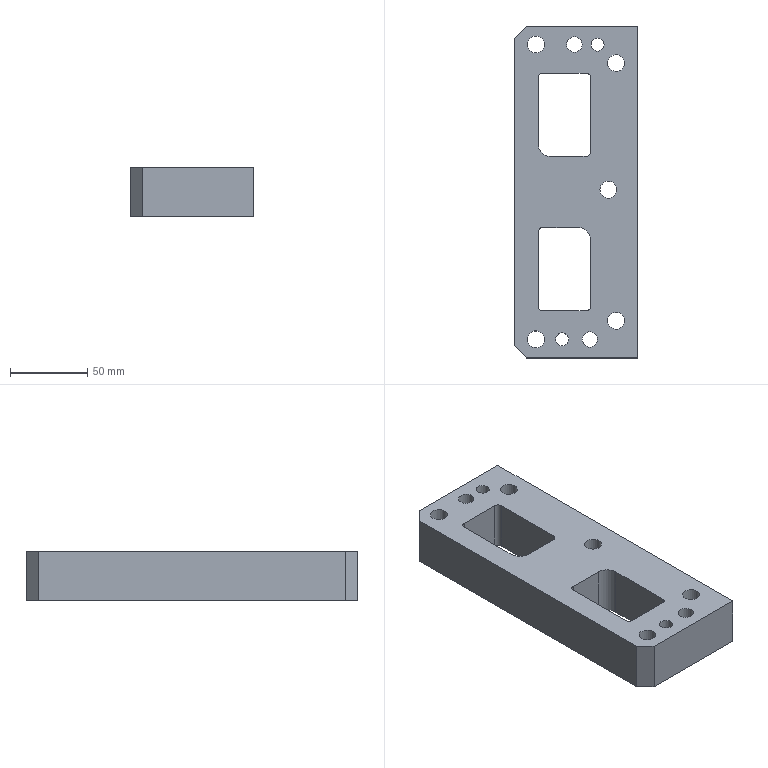Part | STEP file | lll_id3558_x_t | 1 solid | 43 faces | box 80 x 215 x 32 mm | volume 399653 mm3 | cylinder 22 | plane 21 | commonest cylinder face diameters 6 x6 11 x5 17 x5 8.506 x2 10 x2 16 x2
STEP:
#1=CARTESIAN_POINT('',(3684.747,-95.5,60.5));
#2=VERTEX_POINT('',#1);
#3=CARTESIAN_POINT('',(3689.,-95.5,60.5));
#4=DIRECTION('',(0.,0.,1.));
#5=DIRECTION('',(-1.,0.,0.));
#6=AXIS2_PLACEMENT_3D('',#3,#4,#5);
#7=CIRCLE('',#6,4.253);
#8=EDGE_CURVE('',#2,#2,#7,.T.);
#9=ORIENTED_EDGE('',*,*,#8,.T.);
#10=EDGE_LOOP('',(#9));
#11=FACE_BOUND('',#10,.T.);
#12=CARTESIAN_POINT('',(3732.5,-83.5,60.5));
#13=VERTEX_POINT('',#12);
#14=CARTESIAN_POINT('',(3724.,-83.5,60.5));
#15=DIRECTION('',(0.,0.,1.));
#16=DIRECTION('',(1.,0.,0.));
#17=AXIS2_PLACEMENT_3D('',#14,#15,#16);
#18=CIRCLE('',#17,8.5);
#19=EDGE_CURVE('',#13,#13,#18,.T.);
#20=ORIENTED_EDGE('',*,*,#19,.T.);
#21=EDGE_LOOP('',(#20));
#22=FACE_BOUND('',#21,.T.);
#23=CARTESIAN_POINT('',(3680.5,-95.5,60.5));
#24=VERTEX_POINT('',#23);
#25=CARTESIAN_POINT('',(3672.,-95.5,60.5));
#26=DIRECTION('',(0.,0.,1.));
#27=DIRECTION('',(1.,0.,0.));
#28=AXIS2_PLACEMENT_3D('',#25,#26,#27);
#29=CIRCLE('',#28,8.5);
#30=EDGE_CURVE('',#24,#24,#29,.T.);
#31=ORIENTED_EDGE('',*,*,#30,.T.);
#32=EDGE_LOOP('',(#31));
#33=FACE_BOUND('',#32,.T.);
#34=CARTESIAN_POINT('',(3666.,-107.5,60.5));
#35=VERTEX_POINT('',#34);
#36=CARTESIAN_POINT('',(3738.,-107.5,60.5));
#37=VERTEX_POINT('',#36);
#38=CARTESIAN_POINT('',(3700.5,-107.5,60.5));
#39=DIRECTION('',(1.,0.,0.));
#40=VECTOR('',#39,1.);
#41=LINE('',#38,#40);
#42=EDGE_CURVE('',#35,#37,#41,.T.);
#43=ORIENTED_EDGE('',*,*,#42,.F.);
#44=CARTESIAN_POINT('',(3658.,-99.5,60.5));
#45=VERTEX_POINT('',#44);
#46=CARTESIAN_POINT('',(3633.5,-75.,60.5));
#47=DIRECTION('',(-0.7071,0.7071,0.));
#48=VECTOR('',#47,1.);
#49=LINE('',#46,#48);
#50=EDGE_CURVE('',#35,#45,#49,.T.);
#51=ORIENTED_EDGE('',*,*,#50,.T.);
#52=CARTESIAN_POINT('',(3658.,99.5,60.5));
#53=VERTEX_POINT('',#52);
#54=CARTESIAN_POINT('',(3658.,0.00007612,60.5));
#55=DIRECTION('',(0.,-1.,0.));
#56=VECTOR('',#55,1.);
#57=LINE('',#54,#56);
#58=EDGE_CURVE('',#53,#45,#57,.T.);
#59=ORIENTED_EDGE('',*,*,#58,.F.);
#60=CARTESIAN_POINT('',(3666.,107.5,60.5));
#61=VERTEX_POINT('',#60);
#62=CARTESIAN_POINT('',(3633.5,75.,60.5));
#63=DIRECTION('',(0.7071,0.7071,0.));
#64=VECTOR('',#63,1.);
#65=LINE('',#62,#64);
#66=EDGE_CURVE('',#53,#61,#65,.T.);
#67=ORIENTED_EDGE('',*,*,#66,.T.);
#68=CARTESIAN_POINT('',(3738.,107.5,60.5));
#69=VERTEX_POINT('',#68);
#70=CARTESIAN_POINT('',(3700.5,107.5,60.5));
#71=DIRECTION('',(-1.,0.,0.));
#72=VECTOR('',#71,1.);
#73=LINE('',#70,#72);
#74=EDGE_CURVE('',#69,#61,#73,.T.);
#75=ORIENTED_EDGE('',*,*,#74,.F.);
#76=CARTESIAN_POINT('',(3738.,0.00007612,60.5));
#77=DIRECTION('',(0.,1.,0.));
#78=VECTOR('',#77,1.);
#79=LINE('',#76,#78);
#80=EDGE_CURVE('',#37,#69,#79,.T.);
#81=ORIENTED_EDGE('',*,*,#80,.F.);
#82=EDGE_LOOP('',(#43,#51,#59,#67,#75,#81));
#83=FACE_BOUND('',#82,.T.);
#84=CARTESIAN_POINT('',(3732.5,83.5,60.5));
#85=VERTEX_POINT('',#84);
#86=CARTESIAN_POINT('',(3724.,83.5,60.5));
#87=DIRECTION('',(0.,0.,1.));
#88=DIRECTION('',(1.,0.,0.));
#89=AXIS2_PLACEMENT_3D('',#86,#87,#88);
#90=CIRCLE('',#89,8.5);
#91=EDGE_CURVE('',#85,#85,#90,.T.);
#92=ORIENTED_EDGE('',*,*,#91,.T.);
#93=EDGE_LOOP('',(#92));
#94=FACE_BOUND('',#93,.T.);
#95=CARTESIAN_POINT('',(3680.5,95.5,60.5));
#96=VERTEX_POINT('',#95);
#97=CARTESIAN_POINT('',(3672.,95.5,60.5));
#98=DIRECTION('',(0.,0.,1.));
#99=DIRECTION('',(1.,0.,0.));
#100=AXIS2_PLACEMENT_3D('',#97,#98,#99);
#101=CIRCLE('',#100,8.5);
#102=EDGE_CURVE('',#96,#96,#101,.T.);
#103=ORIENTED_EDGE('',*,*,#102,.T.);
#104=EDGE_LOOP('',(#103));
#105=FACE_BOUND('',#104,.T.);
#106=CARTESIAN_POINT('',(3702.,95.5,60.5));
#107=VERTEX_POINT('',#106);
#108=CARTESIAN_POINT('',(3697.,95.5,60.5));
#109=DIRECTION('',(0.,0.,-1.));
#110=DIRECTION('',(1.,0.,0.));
#111=AXIS2_PLACEMENT_3D('',#108,#109,#110);
#112=CIRCLE('',#111,5.);
#113=EDGE_CURVE('',#107,#107,#112,.T.);
#114=ORIENTED_EDGE('',*,*,#113,.F.);
#115=EDGE_LOOP('',(#114));
#116=FACE_BOUND('',#115,.T.);
#117=CARTESIAN_POINT('',(3712.,-95.5,60.5));
#118=VERTEX_POINT('',#117);
#119=CARTESIAN_POINT('',(3707.,-95.5,60.5));
#120=DIRECTION('',(0.,0.,-1.));
#121=DIRECTION('',(1.,0.,0.));
#122=AXIS2_PLACEMENT_3D('',#119,#120,#121);
#123=CIRCLE('',#122,5.);
#124=EDGE_CURVE('',#118,#118,#123,.T.);
#125=ORIENTED_EDGE('',*,*,#124,.F.);
#126=EDGE_LOOP('',(#125));
#127=FACE_BOUND('',#126,.T.);
#128=CARTESIAN_POINT('',(3707.747,95.5,60.5));
#129=VERTEX_POINT('',#128);
#130=CARTESIAN_POINT('',(3712.,95.5,60.5));
#131=DIRECTION('',(0.,0.,1.));
#132=DIRECTION('',(-1.,0.,0.));
#133=AXIS2_PLACEMENT_3D('',#130,#131,#132);
#134=CIRCLE('',#133,4.253);
#135=EDGE_CURVE('',#129,#129,#134,.T.);
#136=ORIENTED_EDGE('',*,*,#135,.T.);
#137=EDGE_LOOP('',(#136));
#138=FACE_BOUND('',#137,.T.);
#139=CARTESIAN_POINT('',(3673.5,31.,60.5));
#140=VERTEX_POINT('',#139);
#141=CARTESIAN_POINT('',(3673.5,74.,60.5));
#142=VERTEX_POINT('',#141);
#143=CARTESIAN_POINT('',(3673.5,28.275,60.5));
#144=DIRECTION('',(0.,1.,0.));
#145=VECTOR('',#144,1.);
#146=LINE('',#143,#145);
#147=EDGE_CURVE('',#140,#142,#146,.T.);
#148=ORIENTED_EDGE('',*,*,#147,.F.);
#149=CARTESIAN_POINT('',(3681.5,23.,60.5));
#150=VERTEX_POINT('',#149);
#151=CARTESIAN_POINT('',(3681.5,31.,60.5));
#152=DIRECTION('',(0.,0.,1.));
#153=DIRECTION('',(1.,0.,0.));
#154=AXIS2_PLACEMENT_3D('',#151,#152,#153);
#155=CIRCLE('',#154,8.);
#156=EDGE_CURVE('',#140,#150,#155,.T.);
#157=ORIENTED_EDGE('',*,*,#156,.T.);
#158=CARTESIAN_POINT('',(3704.5,23.,60.5));
#159=VERTEX_POINT('',#158);
#160=CARTESIAN_POINT('',(3690.5,23.,60.5));
#161=DIRECTION('',(-1.,0.,0.));
#162=VECTOR('',#161,1.);
#163=LINE('',#160,#162);
#164=EDGE_CURVE('',#159,#150,#163,.T.);
#165=ORIENTED_EDGE('',*,*,#164,.F.);
#166=CARTESIAN_POINT('',(3707.5,26.,60.5));
#167=VERTEX_POINT('',#166);
#168=CARTESIAN_POINT('',(3704.5,26.,60.5));
#169=DIRECTION('',(0.,0.,1.));
#170=DIRECTION('',(1.,0.,0.));
#171=AXIS2_PLACEMENT_3D('',#168,#169,#170);
#172=CIRCLE('',#171,3.);
#173=EDGE_CURVE('',#159,#167,#172,.T.);
#174=ORIENTED_EDGE('',*,*,#173,.T.);
#175=CARTESIAN_POINT('',(3707.5,74.,60.5));
#176=VERTEX_POINT('',#175);
#177=CARTESIAN_POINT('',(3707.5,28.275,60.5));
#178=DIRECTION('',(0.,-1.,0.));
#179=VECTOR('',#178,1.);
#180=LINE('',#177,#179);
#181=EDGE_CURVE('',#176,#167,#180,.T.);
#182=ORIENTED_EDGE('',*,*,#181,.F.);
#183=CARTESIAN_POINT('',(3704.5,77.,60.5));
#184=VERTEX_POINT('',#183);
#185=CARTESIAN_POINT('',(3704.5,74.,60.5));
#186=DIRECTION('',(0.,0.,1.));
#187=DIRECTION('',(1.,0.,0.));
#188=AXIS2_PLACEMENT_3D('',#185,#186,#187);
#189=CIRCLE('',#188,3.);
#190=EDGE_CURVE('',#176,#184,#189,.T.);
#191=ORIENTED_EDGE('',*,*,#190,.T.);
#192=CARTESIAN_POINT('',(3676.5,77.,60.5));
#193=VERTEX_POINT('',#192);
#194=CARTESIAN_POINT('',(3690.5,77.,60.5));
#195=DIRECTION('',(1.,0.,0.));
#196=VECTOR('',#195,1.);
#197=LINE('',#194,#196);
#198=EDGE_CURVE('',#193,#184,#197,.T.);
#199=ORIENTED_EDGE('',*,*,#198,.F.);
#200=CARTESIAN_POINT('',(3676.5,74.,60.5));
#201=DIRECTION('',(0.,0.,1.));
#202=DIRECTION('',(1.,0.,0.));
#203=AXIS2_PLACEMENT_3D('',#200,#201,#202);
#204=CIRCLE('',#203,3.);
#205=EDGE_CURVE('',#193,#142,#204,.T.);
#206=ORIENTED_EDGE('',*,*,#205,.T.);
#207=EDGE_LOOP('',(#148,#157,#165,#174,#182,#191,#199,#206));
#208=FACE_BOUND('',#207,.T.);
#209=CARTESIAN_POINT('',(3707.5,-31.,60.5));
#210=VERTEX_POINT('',#209);
#211=CARTESIAN_POINT('',(3707.5,-74.,60.5));
#212=VERTEX_POINT('',#211);
#213=CARTESIAN_POINT('',(3707.5,-28.275,60.5));
#214=DIRECTION('',(0.,-1.,0.));
#215=VECTOR('',#214,1.);
#216=LINE('',#213,#215);
#217=EDGE_CURVE('',#210,#212,#216,.T.);
#218=ORIENTED_EDGE('',*,*,#217,.F.);
#219=CARTESIAN_POINT('',(3699.5,-23.,60.5));
#220=VERTEX_POINT('',#219);
#221=CARTESIAN_POINT('',(3699.5,-31.,60.5));
#222=DIRECTION('',(0.,0.,1.));
#223=DIRECTION('',(1.,0.,0.));
#224=AXIS2_PLACEMENT_3D('',#221,#222,#223);
#225=CIRCLE('',#224,8.);
#226=EDGE_CURVE('',#210,#220,#225,.T.);
#227=ORIENTED_EDGE('',*,*,#226,.T.);
#228=CARTESIAN_POINT('',(3676.5,-23.,60.5));
#229=VERTEX_POINT('',#228);
#230=CARTESIAN_POINT('',(3690.5,-23.,60.5));
#231=DIRECTION('',(1.,0.,0.));
#232=VECTOR('',#231,1.);
#233=LINE('',#230,#232);
#234=EDGE_CURVE('',#229,#220,#233,.T.);
#235=ORIENTED_EDGE('',*,*,#234,.F.);
#236=CARTESIAN_POINT('',(3673.5,-26.,60.5));
#237=VERTEX_POINT('',#236);
#238=CARTESIAN_POINT('',(3676.5,-26.,60.5));
#239=DIRECTION('',(0.,0.,1.));
#240=DIRECTION('',(1.,0.,0.));
#241=AXIS2_PLACEMENT_3D('',#238,#239,#240);
#242=CIRCLE('',#241,3.);
#243=EDGE_CURVE('',#229,#237,#242,.T.);
#244=ORIENTED_EDGE('',*,*,#243,.T.);
#245=CARTESIAN_POINT('',(3673.5,-74.,60.5));
#246=VERTEX_POINT('',#245);
#247=CARTESIAN_POINT('',(3673.5,-28.275,60.5));
#248=DIRECTION('',(0.,1.,0.));
#249=VECTOR('',#248,1.);
#250=LINE('',#247,#249);
#251=EDGE_CURVE('',#246,#237,#250,.T.);
#252=ORIENTED_EDGE('',*,*,#251,.F.);
#253=CARTESIAN_POINT('',(3676.5,-77.,60.5));
#254=VERTEX_POINT('',#253);
#255=CARTESIAN_POINT('',(3676.5,-74.,60.5));
#256=DIRECTION('',(0.,0.,1.));
#257=DIRECTION('',(1.,0.,0.));
#258=AXIS2_PLACEMENT_3D('',#255,#256,#257);
#259=CIRCLE('',#258,3.);
#260=EDGE_CURVE('',#246,#254,#259,.T.);
#261=ORIENTED_EDGE('',*,*,#260,.T.);
#262=CARTESIAN_POINT('',(3704.5,-77.,60.5));
#263=VERTEX_POINT('',#262);
#264=CARTESIAN_POINT('',(3690.5,-77.,60.5));
#265=DIRECTION('',(-1.,0.,0.));
#266=VECTOR('',#265,1.);
#267=LINE('',#264,#266);
#268=EDGE_CURVE('',#263,#254,#267,.T.);
#269=ORIENTED_EDGE('',*,*,#268,.F.);
#270=CARTESIAN_POINT('',(3704.5,-74.,60.5));
#271=DIRECTION('',(0.,0.,1.));
#272=DIRECTION('',(1.,0.,0.));
#273=AXIS2_PLACEMENT_3D('',#270,#271,#272);
#274=CIRCLE('',#273,3.);
#275=EDGE_CURVE('',#263,#212,#274,.T.);
#276=ORIENTED_EDGE('',*,*,#275,.T.);
#277=EDGE_LOOP('',(#218,#227,#235,#244,#252,#261,#269,#276));
#278=FACE_BOUND('',#277,.T.);
#279=CARTESIAN_POINT('',(3727.5,1.5,60.5));
#280=VERTEX_POINT('',#279);
#281=CARTESIAN_POINT('',(3719.,1.5,60.5));
#282=DIRECTION('',(0.,0.,1.));
#283=DIRECTION('',(1.,0.,0.));
#284=AXIS2_PLACEMENT_3D('',#281,#282,#283);
#285=CIRCLE('',#284,8.5);
#286=EDGE_CURVE('',#280,#280,#285,.T.);
#287=ORIENTED_EDGE('',*,*,#286,.T.);
#288=EDGE_LOOP('',(#287));
#289=FACE_BOUND('',#288,.T.);
#290=CARTESIAN_POINT('',(3700.5,0.00007612,60.5));
#291=DIRECTION('',(0.,0.,-1.));
#292=DIRECTION('',(1.,0.,0.));
#293=AXIS2_PLACEMENT_3D('',#290,#291,#292);
#294=PLANE('',#293);
#295=ADVANCED_FACE('',(#11,#22,#33,#83,#94,#105,#116,#127,#138,#208,#278,#289),#294,.T.);
#296=CARTESIAN_POINT('',(3724.5,1.5,92.5));
#297=VERTEX_POINT('',#296);
#298=CARTESIAN_POINT('',(3719.,1.5,92.5));
#299=DIRECTION('',(0.,0.,1.));
#300=DIRECTION('',(1.,0.,0.));
#301=AXIS2_PLACEMENT_3D('',#298,#299,#300);
#302=CIRCLE('',#301,5.5);
#303=EDGE_CURVE('',#297,#297,#302,.T.);
#304=ORIENTED_EDGE('',*,*,#303,.F.);
#305=EDGE_LOOP('',(#304));
#306=FACE_BOUND('',#305,.T.);
#307=CARTESIAN_POINT('',(3699.5,-23.,92.5));
#308=VERTEX_POINT('',#307);
#309=CARTESIAN_POINT('',(3676.5,-23.,92.5));
#310=VERTEX_POINT('',#309);
#311=CARTESIAN_POINT('',(3690.5,-23.,92.5));
#312=DIRECTION('',(-1.,0.,0.));
#313=VECTOR('',#312,1.);
#314=LINE('',#311,#313);
#315=EDGE_CURVE('',#308,#310,#314,.T.);
#316=ORIENTED_EDGE('',*,*,#315,.F.);
#317=CARTESIAN_POINT('',(3707.5,-31.,92.5));
#318=VERTEX_POINT('',#317);
#319=CARTESIAN_POINT('',(3699.5,-31.,92.5));
#320=DIRECTION('',(0.,0.,-1.));
#321=DIRECTION('',(-1.,0.,0.));
#322=AXIS2_PLACEMENT_3D('',#319,#320,#321);
#323=CIRCLE('',#322,8.);
#324=EDGE_CURVE('',#308,#318,#323,.T.);
#325=ORIENTED_EDGE('',*,*,#324,.T.);
#326=CARTESIAN_POINT('',(3707.5,-74.,92.5));
#327=VERTEX_POINT('',#326);
#328=CARTESIAN_POINT('',(3707.5,-28.275,92.5));
#329=DIRECTION('',(0.,1.,0.));
#330=VECTOR('',#329,1.);
#331=LINE('',#328,#330);
#332=EDGE_CURVE('',#327,#318,#331,.T.);
#333=ORIENTED_EDGE('',*,*,#332,.F.);
#334=CARTESIAN_POINT('',(3704.5,-77.,92.5));
#335=VERTEX_POINT('',#334);
#336=CARTESIAN_POINT('',(3704.5,-74.,92.5));
#337=DIRECTION('',(0.,0.,-1.));
#338=DIRECTION('',(-1.,0.,0.));
#339=AXIS2_PLACEMENT_3D('',#336,#337,#338);
#340=CIRCLE('',#339,3.);
#341=EDGE_CURVE('',#327,#335,#340,.T.);
#342=ORIENTED_EDGE('',*,*,#341,.T.);
#343=CARTESIAN_POINT('',(3676.5,-77.,92.5));
#344=VERTEX_POINT('',#343);
#345=CARTESIAN_POINT('',(3690.5,-77.,92.5));
#346=DIRECTION('',(1.,0.,0.));
#347=VECTOR('',#346,1.);
#348=LINE('',#345,#347);
#349=EDGE_CURVE('',#344,#335,#348,.T.);
#350=ORIENTED_EDGE('',*,*,#349,.F.);
#351=CARTESIAN_POINT('',(3673.5,-74.,92.5));
#352=VERTEX_POINT('',#351);
#353=CARTESIAN_POINT('',(3676.5,-74.,92.5));
#354=DIRECTION('',(0.,0.,-1.));
#355=DIRECTION('',(-1.,0.,0.));
#356=AXIS2_PLACEMENT_3D('',#353,#354,#355);
#357=CIRCLE('',#356,3.);
#358=EDGE_CURVE('',#344,#352,#357,.T.);
#359=ORIENTED_EDGE('',*,*,#358,.T.);
#360=CARTESIAN_POINT('',(3673.5,-26.,92.5));
#361=VERTEX_POINT('',#360);
#362=CARTESIAN_POINT('',(3673.5,-28.275,92.5));
#363=DIRECTION('',(0.,-1.,0.));
#364=VECTOR('',#363,1.);
#365=LINE('',#362,#364);
#366=EDGE_CURVE('',#361,#352,#365,.T.);
#367=ORIENTED_EDGE('',*,*,#366,.F.);
#368=CARTESIAN_POINT('',(3676.5,-26.,92.5));
#369=DIRECTION('',(0.,0.,-1.));
#370=DIRECTION('',(-1.,0.,0.));
#371=AXIS2_PLACEMENT_3D('',#368,#369,#370);
#372=CIRCLE('',#371,3.);
#373=EDGE_CURVE('',#361,#310,#372,.T.);
#374=ORIENTED_EDGE('',*,*,#373,.T.);
#375=EDGE_LOOP('',(#316,#325,#333,#342,#350,#359,#367,#374));
#376=FACE_BOUND('',#375,.T.);
#377=CARTESIAN_POINT('',(3681.5,23.,92.5));
#378=VERTEX_POINT('',#377);
#379=CARTESIAN_POINT('',(3704.5,23.,92.5));
#380=VERTEX_POINT('',#379);
#381=CARTESIAN_POINT('',(3690.5,23.,92.5));
#382=DIRECTION('',(1.,0.,0.));
#383=VECTOR('',#382,1.);
#384=LINE('',#381,#383);
#385=EDGE_CURVE('',#378,#380,#384,.T.);
#386=ORIENTED_EDGE('',*,*,#385,.F.);
#387=CARTESIAN_POINT('',(3673.5,31.,92.5));
#388=VERTEX_POINT('',#387);
#389=CARTESIAN_POINT('',(3681.5,31.,92.5));
#390=DIRECTION('',(0.,0.,-1.));
#391=DIRECTION('',(-1.,0.,0.));
#392=AXIS2_PLACEMENT_3D('',#389,#390,#391);
#393=CIRCLE('',#392,8.);
#394=EDGE_CURVE('',#378,#388,#393,.T.);
#395=ORIENTED_EDGE('',*,*,#394,.T.);
#396=CARTESIAN_POINT('',(3673.5,74.,92.5));
#397=VERTEX_POINT('',#396);
#398=CARTESIAN_POINT('',(3673.5,28.275,92.5));
#399=DIRECTION('',(0.,-1.,0.));
#400=VECTOR('',#399,1.);
#401=LINE('',#398,#400);
#402=EDGE_CURVE('',#397,#388,#401,.T.);
#403=ORIENTED_EDGE('',*,*,#402,.F.);
#404=CARTESIAN_POINT('',(3676.5,77.,92.5));
#405=VERTEX_POINT('',#404);
#406=CARTESIAN_POINT('',(3676.5,74.,92.5));
#407=DIRECTION('',(0.,0.,-1.));
#408=DIRECTION('',(-1.,0.,0.));
#409=AXIS2_PLACEMENT_3D('',#406,#407,#408);
#410=CIRCLE('',#409,3.);
#411=EDGE_CURVE('',#397,#405,#410,.T.);
#412=ORIENTED_EDGE('',*,*,#411,.T.);
#413=CARTESIAN_POINT('',(3704.5,77.,92.5));
#414=VERTEX_POINT('',#413);
#415=CARTESIAN_POINT('',(3690.5,77.,92.5));
#416=DIRECTION('',(-1.,0.,0.));
#417=VECTOR('',#416,1.);
#418=LINE('',#415,#417);
#419=EDGE_CURVE('',#414,#405,#418,.T.);
#420=ORIENTED_EDGE('',*,*,#419,.F.);
#421=CARTESIAN_POINT('',(3707.5,74.,92.5));
#422=VERTEX_POINT('',#421);
#423=CARTESIAN_POINT('',(3704.5,74.,92.5));
#424=DIRECTION('',(0.,0.,-1.));
#425=DIRECTION('',(-1.,0.,0.));
#426=AXIS2_PLACEMENT_3D('',#423,#424,#425);
#427=CIRCLE('',#426,3.);
#428=EDGE_CURVE('',#414,#422,#427,.T.);
#429=ORIENTED_EDGE('',*,*,#428,.T.);
#430=CARTESIAN_POINT('',(3707.5,26.,92.5));
#431=VERTEX_POINT('',#430);
#432=CARTESIAN_POINT('',(3707.5,28.275,92.5));
#433=DIRECTION('',(0.,1.,0.));
#434=VECTOR('',#433,1.);
#435=LINE('',#432,#434);
#436=EDGE_CURVE('',#431,#422,#435,.T.);
#437=ORIENTED_EDGE('',*,*,#436,.F.);
#438=CARTESIAN_POINT('',(3704.5,26.,92.5));
#439=DIRECTION('',(0.,0.,-1.));
#440=DIRECTION('',(-1.,0.,0.));
#441=AXIS2_PLACEMENT_3D('',#438,#439,#440);
#442=CIRCLE('',#441,3.);
#443=EDGE_CURVE('',#431,#380,#442,.T.);
#444=ORIENTED_EDGE('',*,*,#443,.T.);
#445=EDGE_LOOP('',(#386,#395,#403,#412,#420,#429,#437,#444));
#446=FACE_BOUND('',#445,.T.);
#447=CARTESIAN_POINT('',(3684.747,-95.5,92.5));
#448=VERTEX_POINT('',#447);
#449=CARTESIAN_POINT('',(3689.,-95.5,92.5));
#450=DIRECTION('',(0.,0.,1.));
#451=DIRECTION('',(-1.,0.,0.));
#452=AXIS2_PLACEMENT_3D('',#449,#450,#451);
#453=CIRCLE('',#452,4.253);
#454=EDGE_CURVE('',#448,#448,#453,.T.);
#455=ORIENTED_EDGE('',*,*,#454,.F.);
#456=EDGE_LOOP('',(#455));
#457=FACE_BOUND('',#456,.T.);
#458=CARTESIAN_POINT('',(3707.747,95.5,92.5));
#459=VERTEX_POINT('',#458);
#460=CARTESIAN_POINT('',(3712.,95.5,92.5));
#461=DIRECTION('',(0.,0.,1.));
#462=DIRECTION('',(-1.,0.,0.));
#463=AXIS2_PLACEMENT_3D('',#460,#461,#462);
#464=CIRCLE('',#463,4.253);
#465=EDGE_CURVE('',#459,#459,#464,.T.);
#466=ORIENTED_EDGE('',*,*,#465,.F.);
#467=EDGE_LOOP('',(#466));
#468=FACE_BOUND('',#467,.T.);
#469=CARTESIAN_POINT('',(3702.,-95.5,92.5));
#470=VERTEX_POINT('',#469);
#471=CARTESIAN_POINT('',(3707.,-95.5,92.5));
#472=DIRECTION('',(0.,0.,1.));
#473=DIRECTION('',(-1.,0.,0.));
#474=AXIS2_PLACEMENT_3D('',#471,#472,#473);
#475=CIRCLE('',#474,5.);
#476=EDGE_CURVE('',#470,#470,#475,.T.);
#477=ORIENTED_EDGE('',*,*,#476,.F.);
#478=EDGE_LOOP('',(#477));
#479=FACE_BOUND('',#478,.T.);
#480=CARTESIAN_POINT('',(3692.,95.5,92.5));
#481=VERTEX_POINT('',#480);
#482=CARTESIAN_POINT('',(3697.,95.5,92.5));
#483=DIRECTION('',(0.,0.,1.));
#484=DIRECTION('',(-1.,0.,0.));
#485=AXIS2_PLACEMENT_3D('',#482,#483,#484);
#486=CIRCLE('',#485,5.);
#487=EDGE_CURVE('',#481,#481,#486,.T.);
#488=ORIENTED_EDGE('',*,*,#487,.F.);
#489=EDGE_LOOP('',(#488));
#490=FACE_BOUND('',#489,.T.);
#491=CARTESIAN_POINT('',(3718.5,-83.5,92.5));
#492=VERTEX_POINT('',#491);
#493=CARTESIAN_POINT('',(3724.,-83.5,92.5));
#494=DIRECTION('',(0.,0.,1.));
#495=DIRECTION('',(-1.,0.,0.));
#496=AXIS2_PLACEMENT_3D('',#493,#494,#495);
#497=CIRCLE('',#496,5.5);
#498=EDGE_CURVE('',#492,#492,#497,.T.);
#499=ORIENTED_EDGE('',*,*,#498,.F.);
#500=EDGE_LOOP('',(#499));
#501=FACE_BOUND('',#500,.T.);
#502=CARTESIAN_POINT('',(3666.5,95.5,92.5));
#503=VERTEX_POINT('',#502);
#504=CARTESIAN_POINT('',(3672.,95.5,92.5));
#505=DIRECTION('',(0.,0.,1.));
#506=DIRECTION('',(-1.,0.,0.));
#507=AXIS2_PLACEMENT_3D('',#504,#505,#506);
#508=CIRCLE('',#507,5.5);
#509=EDGE_CURVE('',#503,#503,#508,.T.);
#510=ORIENTED_EDGE('',*,*,#509,.F.);
#511=EDGE_LOOP('',(#510));
#512=FACE_BOUND('',#511,.T.);
#513=CARTESIAN_POINT('',(3666.5,-95.5,92.5));
#514=VERTEX_POINT('',#513);
#515=CARTESIAN_POINT('',(3672.,-95.5,92.5));
#516=DIRECTION('',(0.,0.,1.));
#517=DIRECTION('',(-1.,0.,0.));
#518=AXIS2_PLACEMENT_3D('',#515,#516,#517);
#519=CIRCLE('',#518,5.5);
#520=EDGE_CURVE('',#514,#514,#519,.T.);
#521=ORIENTED_EDGE('',*,*,#520,.F.);
#522=EDGE_LOOP('',(#521));
#523=FACE_BOUND('',#522,.T.);
#524=CARTESIAN_POINT('',(3718.5,83.5,92.5));
#525=VERTEX_POINT('',#524);
#526=CARTESIAN_POINT('',(3724.,83.5,92.5));
#527=DIRECTION('',(0.,0.,1.));
#528=DIRECTION('',(-1.,0.,0.));
#529=AXIS2_PLACEMENT_3D('',#526,#527,#528);
#530=CIRCLE('',#529,5.5);
#531=EDGE_CURVE('',#525,#525,#530,.T.);
#532=ORIENTED_EDGE('',*,*,#531,.F.);
#533=EDGE_LOOP('',(#532));
#534=FACE_BOUND('',#533,.T.);
#535=CARTESIAN_POINT('',(3658.,-99.5,92.5));
#536=VERTEX_POINT('',#535);
#537=CARTESIAN_POINT('',(3658.,99.5,92.5));
#538=VERTEX_POINT('',#537);
#539=CARTESIAN_POINT('',(3658.,0.00007612,92.5));
#540=DIRECTION('',(0.,1.,0.));
#541=VECTOR('',#540,1.);
#542=LINE('',#539,#541);
#543=EDGE_CURVE('',#536,#538,#542,.T.);
#544=ORIENTED_EDGE('',*,*,#543,.F.);
#545=CARTESIAN_POINT('',(3666.,-107.5,92.5));
#546=VERTEX_POINT('',#545);
#547=CARTESIAN_POINT('',(3633.5,-75.,92.5));
#548=DIRECTION('',(0.7071,-0.7071,0.));
#549=VECTOR('',#548,1.);
#550=LINE('',#547,#549);
#551=EDGE_CURVE('',#536,#546,#550,.T.);
#552=ORIENTED_EDGE('',*,*,#551,.T.);
#553=CARTESIAN_POINT('',(3738.,-107.5,92.5));
#554=VERTEX_POINT('',#553);
#555=CARTESIAN_POINT('',(3700.5,-107.5,92.5));
#556=DIRECTION('',(-1.,0.,0.));
#557=VECTOR('',#556,1.);
#558=LINE('',#555,#557);
#559=EDGE_CURVE('',#554,#546,#558,.T.);
#560=ORIENTED_EDGE('',*,*,#559,.F.);
#561=CARTESIAN_POINT('',(3738.,107.5,92.5));
#562=VERTEX_POINT('',#561);
#563=CARTESIAN_POINT('',(3738.,0.00007612,92.5));
#564=DIRECTION('',(0.,-1.,0.));
#565=VECTOR('',#564,1.);
#566=LINE('',#563,#565);
#567=EDGE_CURVE('',#562,#554,#566,.T.);
#568=ORIENTED_EDGE('',*,*,#567,.F.);
#569=CARTESIAN_POINT('',(3666.,107.5,92.5));
#570=VERTEX_POINT('',#569);
#571=CARTESIAN_POINT('',(3700.5,107.5,92.5));
#572=DIRECTION('',(1.,0.,0.));
#573=VECTOR('',#572,1.);
#574=LINE('',#571,#573);
#575=EDGE_CURVE('',#570,#562,#574,.T.);
#576=ORIENTED_EDGE('',*,*,#575,.F.);
#577=CARTESIAN_POINT('',(3633.5,75.,92.5));
#578=DIRECTION('',(-0.7071,-0.7071,0.));
#579=VECTOR('',#578,1.);
#580=LINE('',#577,#579);
#581=EDGE_CURVE('',#570,#538,#580,.T.);
#582=ORIENTED_EDGE('',*,*,#581,.T.);
#583=EDGE_LOOP('',(#544,#552,#560,#568,#576,#582));
#584=FACE_BOUND('',#583,.T.);
#585=CARTESIAN_POINT('',(3700.5,0.00007612,92.5));
#586=DIRECTION('',(0.,0.,1.));
#587=DIRECTION('',(-1.,0.,0.));
#588=AXIS2_PLACEMENT_3D('',#585,#586,#587);
#589=PLANE('',#588);
#590=ADVANCED_FACE('',(#306,#376,#446,#457,#468,#479,#490,#501,#512,#523,#534,#584),#589,.T.);
#591=ORIENTED_EDGE('',*,*,#74,.T.);
#592=CARTESIAN_POINT('',(3666.,107.5,60.5));
#593=DIRECTION('',(0.,0.,1.));
#594=VECTOR('',#593,1.);
#595=LINE('',#592,#594);
#596=EDGE_CURVE('',#61,#570,#595,.T.);
#597=ORIENTED_EDGE('',*,*,#596,.T.);
#598=ORIENTED_EDGE('',*,*,#575,.T.);
#599=CARTESIAN_POINT('',(3738.,107.5,60.5));
#600=DIRECTION('',(0.,0.,1.));
#601=VECTOR('',#600,1.);
#602=LINE('',#599,#601);
#603=EDGE_CURVE('',#69,#562,#602,.T.);
#604=ORIENTED_EDGE('',*,*,#603,.F.);
#605=EDGE_LOOP('',(#591,#597,#598,#604));
#606=FACE_OUTER_BOUND('',#605,.T.);
#607=CARTESIAN_POINT('',(3700.5,107.5,60.5));
#608=DIRECTION('',(0.,1.,0.));
#609=DIRECTION('',(0.,0.,-1.));
#610=AXIS2_PLACEMENT_3D('',#607,#608,#609);
#611=PLANE('',#610);
#612=ADVANCED_FACE('',(#606),#611,.T.);
#613=ORIENTED_EDGE('',*,*,#603,.T.);
#614=ORIENTED_EDGE('',*,*,#567,.T.);
#615=CARTESIAN_POINT('',(3738.,-107.5,60.5));
#616=DIRECTION('',(0.,0.,1.));
#617=VECTOR('',#616,1.);
#618=LINE('',#615,#617);
#619=EDGE_CURVE('',#37,#554,#618,.T.);
#620=ORIENTED_EDGE('',*,*,#619,.F.);
#621=ORIENTED_EDGE('',*,*,#80,.T.);
#622=EDGE_LOOP('',(#613,#614,#620,#621));
#623=FACE_OUTER_BOUND('',#622,.T.);
#624=CARTESIAN_POINT('',(3738.,0.00007612,60.5));
#625=DIRECTION('',(1.,0.,0.));
#626=DIRECTION('',(0.,0.,1.));
#627=AXIS2_PLACEMENT_3D('',#624,#625,#626);
#628=PLANE('',#627);
#629=ADVANCED_FACE('',(#623),#628,.T.);
#630=ORIENTED_EDGE('',*,*,#559,.T.);
#631=CARTESIAN_POINT('',(3666.,-107.5,60.5));
#632=DIRECTION('',(0.,0.,-1.));
#633=VECTOR('',#632,1.);
#634=LINE('',#631,#633);
#635=EDGE_CURVE('',#546,#35,#634,.T.);
#636=ORIENTED_EDGE('',*,*,#635,.T.);
#637=ORIENTED_EDGE('',*,*,#42,.T.);
#638=ORIENTED_EDGE('',*,*,#619,.T.);
#639=EDGE_LOOP('',(#630,#636,#637,#638));
#640=FACE_OUTER_BOUND('',#639,.T.);
#641=CARTESIAN_POINT('',(3700.5,-107.5,60.5));
#642=DIRECTION('',(0.,-1.,0.));
#643=DIRECTION('',(0.,0.,1.));
#644=AXIS2_PLACEMENT_3D('',#641,#642,#643);
#645=PLANE('',#644);
#646=ADVANCED_FACE('',(#640),#645,.T.);
#647=ORIENTED_EDGE('',*,*,#58,.T.);
#648=CARTESIAN_POINT('',(3658.,-99.5,60.5));
#649=DIRECTION('',(0.,0.,1.));
#650=VECTOR('',#649,1.);
#651=LINE('',#648,#650);
#652=EDGE_CURVE('',#45,#536,#651,.T.);
#653=ORIENTED_EDGE('',*,*,#652,.T.);
#654=ORIENTED_EDGE('',*,*,#543,.T.);
#655=CARTESIAN_POINT('',(3658.,99.5,60.5));
#656=DIRECTION('',(0.,0.,-1.));
#657=VECTOR('',#656,1.);
#658=LINE('',#655,#657);
#659=EDGE_CURVE('',#538,#53,#658,.T.);
#660=ORIENTED_EDGE('',*,*,#659,.T.);
#661=EDGE_LOOP('',(#647,#653,#654,#660));
#662=FACE_OUTER_BOUND('',#661,.T.);
#663=CARTESIAN_POINT('',(3658.,0.00007612,60.5));
#664=DIRECTION('',(-1.,0.,0.));
#665=DIRECTION('',(0.,0.,-1.));
#666=AXIS2_PLACEMENT_3D('',#663,#664,#665);
#667=PLANE('',#666);
#668=ADVANCED_FACE('',(#662),#667,.T.);
#669=ORIENTED_EDGE('',*,*,#531,.T.);
#670=EDGE_LOOP('',(#669));
#671=FACE_BOUND('',#670,.T.);
#672=CARTESIAN_POINT('',(3718.5,83.5,73.5));
#673=VERTEX_POINT('',#672);
#674=CARTESIAN_POINT('',(3724.,83.5,73.5));
#675=DIRECTION('',(0.,0.,1.));
#676=DIRECTION('',(-1.,0.,0.));
#677=AXIS2_PLACEMENT_3D('',#674,#675,#676);
#678=CIRCLE('',#677,5.5);
#679=EDGE_CURVE('',#673,#673,#678,.T.);
#680=ORIENTED_EDGE('',*,*,#679,.F.);
#681=EDGE_LOOP('',(#680));
#682=FACE_BOUND('',#681,.T.);
#683=CARTESIAN_POINT('',(3724.,83.5,57.5));
#684=DIRECTION('',(0.,0.,1.));
#685=DIRECTION('',(-1.,0.,0.));
#686=AXIS2_PLACEMENT_3D('',#683,#684,#685);
#687=CYLINDRICAL_SURFACE('',#686,5.5);
#688=ADVANCED_FACE('',(#671,#682),#687,.F.);
#689=ORIENTED_EDGE('',*,*,#679,.T.);
#690=EDGE_LOOP('',(#689));
#691=FACE_BOUND('',#690,.T.);
#692=CARTESIAN_POINT('',(3715.5,83.5,73.5));
#693=VERTEX_POINT('',#692);
#694=CARTESIAN_POINT('',(3724.,83.5,73.5));
#695=DIRECTION('',(0.,0.,1.));
#696=DIRECTION('',(-1.,0.,0.));
#697=AXIS2_PLACEMENT_3D('',#694,#695,#696);
#698=CIRCLE('',#697,8.5);
#699=EDGE_CURVE('',#693,#693,#698,.T.);
#700=ORIENTED_EDGE('',*,*,#699,.F.);
#701=EDGE_LOOP('',(#700));
#702=FACE_BOUND('',#701,.T.);
#703=CARTESIAN_POINT('',(3724.,83.5,73.5));
#704=DIRECTION('',(0.,0.,1.));
#705=DIRECTION('',(-1.,0.,0.));
#706=AXIS2_PLACEMENT_3D('',#703,#704,#705);
#707=PLANE('',#706);
#708=ADVANCED_FACE('',(#691,#702),#707,.F.);
#709=ORIENTED_EDGE('',*,*,#699,.T.);
#710=EDGE_LOOP('',(#709));
#711=FACE_BOUND('',#710,.T.);
#712=ORIENTED_EDGE('',*,*,#91,.F.);
#713=EDGE_LOOP('',(#712));
#714=FACE_BOUND('',#713,.T.);
#715=CARTESIAN_POINT('',(3724.,83.5,60.5));
#716=DIRECTION('',(0.,0.,1.));
#717=DIRECTION('',(-1.,0.,0.));
#718=AXIS2_PLACEMENT_3D('',#715,#716,#717);
#719=CYLINDRICAL_SURFACE('',#718,8.5);
#720=ADVANCED_FACE('',(#711,#714),#719,.F.);
#721=ORIENTED_EDGE('',*,*,#520,.T.);
#722=EDGE_LOOP('',(#721));
#723=FACE_BOUND('',#722,.T.);
#724=CARTESIAN_POINT('',(3666.5,-95.5,73.5));
#725=VERTEX_POINT('',#724);
#726=CARTESIAN_POINT('',(3672.,-95.5,73.5));
#727=DIRECTION('',(0.,0.,1.));
#728=DIRECTION('',(-1.,0.,0.));
#729=AXIS2_PLACEMENT_3D('',#726,#727,#728);
#730=CIRCLE('',#729,5.5);
#731=EDGE_CURVE('',#725,#725,#730,.T.);
#732=ORIENTED_EDGE('',*,*,#731,.F.);
#733=EDGE_LOOP('',(#732));
#734=FACE_BOUND('',#733,.T.);
#735=CARTESIAN_POINT('',(3672.,-95.5,57.5));
#736=DIRECTION('',(0.,0.,1.));
#737=DIRECTION('',(-1.,0.,0.));
#738=AXIS2_PLACEMENT_3D('',#735,#736,#737);
#739=CYLINDRICAL_SURFACE('',#738,5.5);
#740=ADVANCED_FACE('',(#723,#734),#739,.F.);
#741=ORIENTED_EDGE('',*,*,#731,.T.);
#742=EDGE_LOOP('',(#741));
#743=FACE_BOUND('',#742,.T.);
#744=CARTESIAN_POINT('',(3663.5,-95.5,73.5));
#745=VERTEX_POINT('',#744);
#746=CARTESIAN_POINT('',(3672.,-95.5,73.5));
#747=DIRECTION('',(0.,0.,1.));
#748=DIRECTION('',(-1.,0.,0.));
#749=AXIS2_PLACEMENT_3D('',#746,#747,#748);
#750=CIRCLE('',#749,8.5);
#751=EDGE_CURVE('',#745,#745,#750,.T.);
#752=ORIENTED_EDGE('',*,*,#751,.F.);
#753=EDGE_LOOP('',(#752));
#754=FACE_BOUND('',#753,.T.);
#755=CARTESIAN_POINT('',(3672.,-95.5,73.5));
#756=DIRECTION('',(0.,0.,1.));
#757=DIRECTION('',(-1.,0.,0.));
#758=AXIS2_PLACEMENT_3D('',#755,#756,#757);
#759=PLANE('',#758);
#760=ADVANCED_FACE('',(#743,#754),#759,.F.);
#761=ORIENTED_EDGE('',*,*,#751,.T.);
#762=EDGE_LOOP('',(#761));
#763=FACE_BOUND('',#762,.T.);
#764=ORIENTED_EDGE('',*,*,#30,.F.);
#765=EDGE_LOOP('',(#764));
#766=FACE_BOUND('',#765,.T.);
#767=CARTESIAN_POINT('',(3672.,-95.5,60.5));
#768=DIRECTION('',(0.,0.,1.));
#769=DIRECTION('',(-1.,0.,0.));
#770=AXIS2_PLACEMENT_3D('',#767,#768,#769);
#771=CYLINDRICAL_SURFACE('',#770,8.5);
#772=ADVANCED_FACE('',(#763,#766),#771,.F.);
#773=ORIENTED_EDGE('',*,*,#509,.T.);
#774=EDGE_LOOP('',(#773));
#775=FACE_BOUND('',#774,.T.);
#776=CARTESIAN_POINT('',(3666.5,95.5,73.5));
#777=VERTEX_POINT('',#776);
#778=CARTESIAN_POINT('',(3672.,95.5,73.5));
#779=DIRECTION('',(0.,0.,1.));
#780=DIRECTION('',(-1.,0.,0.));
#781=AXIS2_PLACEMENT_3D('',#778,#779,#780);
#782=CIRCLE('',#781,5.5);
#783=EDGE_CURVE('',#777,#777,#782,.T.);
#784=ORIENTED_EDGE('',*,*,#783,.F.);
#785=EDGE_LOOP('',(#784));
#786=FACE_BOUND('',#785,.T.);
#787=CARTESIAN_POINT('',(3672.,95.5,57.5));
#788=DIRECTION('',(0.,0.,1.));
#789=DIRECTION('',(-1.,0.,0.));
#790=AXIS2_PLACEMENT_3D('',#787,#788,#789);
#791=CYLINDRICAL_SURFACE('',#790,5.5);
#792=ADVANCED_FACE('',(#775,#786),#791,.F.);
#793=ORIENTED_EDGE('',*,*,#783,.T.);
#794=EDGE_LOOP('',(#793));
#795=FACE_BOUND('',#794,.T.);
#796=CARTESIAN_POINT('',(3663.5,95.5,73.5));
#797=VERTEX_POINT('',#796);
#798=CARTESIAN_POINT('',(3672.,95.5,73.5));
#799=DIRECTION('',(0.,0.,1.));
#800=DIRECTION('',(-1.,0.,0.));
#801=AXIS2_PLACEMENT_3D('',#798,#799,#800);
#802=CIRCLE('',#801,8.5);
#803=EDGE_CURVE('',#797,#797,#802,.T.);
#804=ORIENTED_EDGE('',*,*,#803,.F.);
#805=EDGE_LOOP('',(#804));
#806=FACE_BOUND('',#805,.T.);
#807=CARTESIAN_POINT('',(3672.,95.5,73.5));
#808=DIRECTION('',(0.,0.,1.));
#809=DIRECTION('',(-1.,0.,0.));
#810=AXIS2_PLACEMENT_3D('',#807,#808,#809);
#811=PLANE('',#810);
#812=ADVANCED_FACE('',(#795,#806),#811,.F.);
#813=ORIENTED_EDGE('',*,*,#803,.T.);
#814=EDGE_LOOP('',(#813));
#815=FACE_BOUND('',#814,.T.);
#816=ORIENTED_EDGE('',*,*,#102,.F.);
#817=EDGE_LOOP('',(#816));
#818=FACE_BOUND('',#817,.T.);
#819=CARTESIAN_POINT('',(3672.,95.5,60.5));
#820=DIRECTION('',(0.,0.,1.));
#821=DIRECTION('',(-1.,0.,0.));
#822=AXIS2_PLACEMENT_3D('',#819,#820,#821);
#823=CYLINDRICAL_SURFACE('',#822,8.5);
#824=ADVANCED_FACE('',(#815,#818),#823,.F.);
#825=ORIENTED_EDGE('',*,*,#498,.T.);
#826=EDGE_LOOP('',(#825));
#827=FACE_BOUND('',#826,.T.);
#828=CARTESIAN_POINT('',(3718.5,-83.5,73.5));
#829=VERTEX_POINT('',#828);
#830=CARTESIAN_POINT('',(3724.,-83.5,73.5));
#831=DIRECTION('',(0.,0.,1.));
#832=DIRECTION('',(-1.,0.,0.));
#833=AXIS2_PLACEMENT_3D('',#830,#831,#832);
#834=CIRCLE('',#833,5.5);
#835=EDGE_CURVE('',#829,#829,#834,.T.);
#836=ORIENTED_EDGE('',*,*,#835,.F.);
#837=EDGE_LOOP('',(#836));
#838=FACE_BOUND('',#837,.T.);
#839=CARTESIAN_POINT('',(3724.,-83.5,57.5));
#840=DIRECTION('',(0.,0.,1.));
#841=DIRECTION('',(-1.,0.,0.));
#842=AXIS2_PLACEMENT_3D('',#839,#840,#841);
#843=CYLINDRICAL_SURFACE('',#842,5.5);
#844=ADVANCED_FACE('',(#827,#838),#843,.F.);
#845=ORIENTED_EDGE('',*,*,#835,.T.);
#846=EDGE_LOOP('',(#845));
#847=FACE_BOUND('',#846,.T.);
#848=CARTESIAN_POINT('',(3715.5,-83.5,73.5));
#849=VERTEX_POINT('',#848);
#850=CARTESIAN_POINT('',(3724.,-83.5,73.5));
#851=DIRECTION('',(0.,0.,1.));
#852=DIRECTION('',(-1.,0.,0.));
#853=AXIS2_PLACEMENT_3D('',#850,#851,#852);
#854=CIRCLE('',#853,8.5);
#855=EDGE_CURVE('',#849,#849,#854,.T.);
#856=ORIENTED_EDGE('',*,*,#855,.F.);
#857=EDGE_LOOP('',(#856));
#858=FACE_BOUND('',#857,.T.);
#859=CARTESIAN_POINT('',(3724.,-83.5,73.5));
#860=DIRECTION('',(0.,0.,1.));
#861=DIRECTION('',(-1.,0.,0.));
#862=AXIS2_PLACEMENT_3D('',#859,#860,#861);
#863=PLANE('',#862);
#864=ADVANCED_FACE('',(#847,#858),#863,.F.);
#865=ORIENTED_EDGE('',*,*,#855,.T.);
#866=EDGE_LOOP('',(#865));
#867=FACE_BOUND('',#866,.T.);
#868=ORIENTED_EDGE('',*,*,#19,.F.);
#869=EDGE_LOOP('',(#868));
#870=FACE_BOUND('',#869,.T.);
#871=CARTESIAN_POINT('',(3724.,-83.5,60.5));
#872=DIRECTION('',(0.,0.,1.));
#873=DIRECTION('',(-1.,0.,0.));
#874=AXIS2_PLACEMENT_3D('',#871,#872,#873);
#875=CYLINDRICAL_SURFACE('',#874,8.5);
#876=ADVANCED_FACE('',(#867,#870),#875,.F.);
#877=ORIENTED_EDGE('',*,*,#113,.T.);
#878=EDGE_LOOP('',(#877));
#879=FACE_BOUND('',#878,.T.);
#880=ORIENTED_EDGE('',*,*,#487,.T.);
#881=EDGE_LOOP('',(#880));
#882=FACE_BOUND('',#881,.T.);
#883=CARTESIAN_POINT('',(3697.,95.5,57.5));
#884=DIRECTION('',(0.,0.,1.));
#885=DIRECTION('',(-1.,0.,0.));
#886=AXIS2_PLACEMENT_3D('',#883,#884,#885);
#887=CYLINDRICAL_SURFACE('',#886,5.);
#888=ADVANCED_FACE('',(#879,#882),#887,.F.);
#889=ORIENTED_EDGE('',*,*,#124,.T.);
#890=EDGE_LOOP('',(#889));
#891=FACE_BOUND('',#890,.T.);
#892=ORIENTED_EDGE('',*,*,#476,.T.);
#893=EDGE_LOOP('',(#892));
#894=FACE_BOUND('',#893,.T.);
#895=CARTESIAN_POINT('',(3707.,-95.5,57.5));
#896=DIRECTION('',(0.,0.,1.));
#897=DIRECTION('',(-1.,0.,0.));
#898=AXIS2_PLACEMENT_3D('',#895,#896,#897);
#899=CYLINDRICAL_SURFACE('',#898,5.);
#900=ADVANCED_FACE('',(#891,#894),#899,.F.);
#901=ORIENTED_EDGE('',*,*,#465,.T.);
#902=EDGE_LOOP('',(#901));
#903=FACE_BOUND('',#902,.T.);
#904=ORIENTED_EDGE('',*,*,#135,.F.);
#905=EDGE_LOOP('',(#904));
#906=FACE_BOUND('',#905,.T.);
#907=CARTESIAN_POINT('',(3712.,95.5,60.5));
#908=DIRECTION('',(0.,0.,1.));
#909=DIRECTION('',(-1.,0.,0.));
#910=AXIS2_PLACEMENT_3D('',#907,#908,#909);
#911=CYLINDRICAL_SURFACE('',#910,4.253);
#912=ADVANCED_FACE('',(#903,#906),#911,.F.);
#913=ORIENTED_EDGE('',*,*,#454,.T.);
#914=EDGE_LOOP('',(#913));
#915=FACE_BOUND('',#914,.T.);
#916=ORIENTED_EDGE('',*,*,#8,.F.);
#917=EDGE_LOOP('',(#916));
#918=FACE_BOUND('',#917,.T.);
#919=CARTESIAN_POINT('',(3689.,-95.5,60.5));
#920=DIRECTION('',(0.,0.,1.));
#921=DIRECTION('',(-1.,0.,0.));
#922=AXIS2_PLACEMENT_3D('',#919,#920,#921);
#923=CYLINDRICAL_SURFACE('',#922,4.253);
#924=ADVANCED_FACE('',(#915,#918),#923,.F.);
#925=ORIENTED_EDGE('',*,*,#402,.T.);
#926=CARTESIAN_POINT('',(3673.5,31.,60.5));
#927=DIRECTION('',(0.,0.,-1.));
#928=VECTOR('',#927,1.);
#929=LINE('',#926,#928);
#930=EDGE_CURVE('',#388,#140,#929,.T.);
#931=ORIENTED_EDGE('',*,*,#930,.T.);
#932=ORIENTED_EDGE('',*,*,#147,.T.);
#933=CARTESIAN_POINT('',(3673.5,74.,92.5));
#934=DIRECTION('',(0.,0.,1.));
#935=VECTOR('',#934,1.);
#936=LINE('',#933,#935);
#937=EDGE_CURVE('',#142,#397,#936,.T.);
#938=ORIENTED_EDGE('',*,*,#937,.T.);
#939=EDGE_LOOP('',(#925,#931,#932,#938));
#940=FACE_OUTER_BOUND('',#939,.T.);
#941=CARTESIAN_POINT('',(3673.5,59.5,-8.5));
#942=DIRECTION('',(-1.,0.,0.));
#943=DIRECTION('',(0.,0.,1.));
#944=AXIS2_PLACEMENT_3D('',#941,#942,#943);
#945=PLANE('',#944);
#946=ADVANCED_FACE('',(#940),#945,.F.);
#947=ORIENTED_EDGE('',*,*,#198,.T.);
#948=CARTESIAN_POINT('',(3704.5,77.,92.5));
#949=DIRECTION('',(0.,0.,1.));
#950=VECTOR('',#949,1.);
#951=LINE('',#948,#950);
#952=EDGE_CURVE('',#184,#414,#951,.T.);
#953=ORIENTED_EDGE('',*,*,#952,.T.);
#954=ORIENTED_EDGE('',*,*,#419,.T.);
#955=CARTESIAN_POINT('',(3676.5,77.,60.5));
#956=DIRECTION('',(0.,0.,-1.));
#957=VECTOR('',#956,1.);
#958=LINE('',#955,#957);
#959=EDGE_CURVE('',#405,#193,#958,.T.);
#960=ORIENTED_EDGE('',*,*,#959,.T.);
#961=EDGE_LOOP('',(#947,#953,#954,#960));
#962=FACE_OUTER_BOUND('',#961,.T.);
#963=CARTESIAN_POINT('',(3690.5,77.,-8.5));
#964=DIRECTION('',(0.,1.,0.));
#965=DIRECTION('',(0.,0.,-1.));
#966=AXIS2_PLACEMENT_3D('',#963,#964,#965);
#967=PLANE('',#966);
#968=ADVANCED_FACE('',(#962),#967,.F.);
#969=ORIENTED_EDGE('',*,*,#181,.T.);
#970=CARTESIAN_POINT('',(3707.5,26.,92.5));
#971=DIRECTION('',(0.,0.,1.));
#972=VECTOR('',#971,1.);
#973=LINE('',#970,#972);
#974=EDGE_CURVE('',#167,#431,#973,.T.);
#975=ORIENTED_EDGE('',*,*,#974,.T.);
#976=ORIENTED_EDGE('',*,*,#436,.T.);
#977=CARTESIAN_POINT('',(3707.5,74.,60.5));
#978=DIRECTION('',(0.,0.,-1.));
#979=VECTOR('',#978,1.);
#980=LINE('',#977,#979);
#981=EDGE_CURVE('',#422,#176,#980,.T.);
#982=ORIENTED_EDGE('',*,*,#981,.T.);
#983=EDGE_LOOP('',(#969,#975,#976,#982));
#984=FACE_OUTER_BOUND('',#983,.T.);
#985=CARTESIAN_POINT('',(3707.5,59.5,-8.5));
#986=DIRECTION('',(1.,0.,0.));
#987=DIRECTION('',(0.,0.,-1.));
#988=AXIS2_PLACEMENT_3D('',#985,#986,#987);
#989=PLANE('',#988);
#990=ADVANCED_FACE('',(#984),#989,.F.);
#991=ORIENTED_EDGE('',*,*,#164,.T.);
#992=CARTESIAN_POINT('',(3681.5,23.,92.5));
#993=DIRECTION('',(0.,0.,1.));
#994=VECTOR('',#993,1.);
#995=LINE('',#992,#994);
#996=EDGE_CURVE('',#150,#378,#995,.T.);
#997=ORIENTED_EDGE('',*,*,#996,.T.);
#998=ORIENTED_EDGE('',*,*,#385,.T.);
#999=CARTESIAN_POINT('',(3704.5,23.,60.5));
#1000=DIRECTION('',(0.,0.,-1.));
#1001=VECTOR('',#1000,1.);
#1002=LINE('',#999,#1001);
#1003=EDGE_CURVE('',#380,#159,#1002,.T.);
#1004=ORIENTED_EDGE('',*,*,#1003,.T.);
#1005=EDGE_LOOP('',(#991,#997,#998,#1004));
#1006=FACE_OUTER_BOUND('',#1005,.T.);
#1007=CARTESIAN_POINT('',(3690.5,23.,-8.5));
#1008=DIRECTION('',(0.,-1.,0.));
#1009=DIRECTION('',(0.,0.,1.));
#1010=AXIS2_PLACEMENT_3D('',#1007,#1008,#1009);
#1011=PLANE('',#1010);
#1012=ADVANCED_FACE('',(#1006),#1011,.F.);
#1013=ORIENTED_EDGE('',*,*,#332,.T.);
#1014=CARTESIAN_POINT('',(3707.5,-31.,60.5));
#1015=DIRECTION('',(0.,0.,-1.));
#1016=VECTOR('',#1015,1.);
#1017=LINE('',#1014,#1016);
#1018=EDGE_CURVE('',#318,#210,#1017,.T.);
#1019=ORIENTED_EDGE('',*,*,#1018,.T.);
#1020=ORIENTED_EDGE('',*,*,#217,.T.);
#1021=CARTESIAN_POINT('',(3707.5,-74.,92.5));
#1022=DIRECTION('',(0.,0.,1.));
#1023=VECTOR('',#1022,1.);
#1024=LINE('',#1021,#1023);
#1025=EDGE_CURVE('',#212,#327,#1024,.T.);
#1026=ORIENTED_EDGE('',*,*,#1025,.T.);
#1027=EDGE_LOOP('',(#1013,#1019,#1020,#1026));
#1028=FACE_OUTER_BOUND('',#1027,.T.);
#1029=CARTESIAN_POINT('',(3707.5,-59.5,-8.5));
#1030=DIRECTION('',(1.,0.,0.));
#1031=DIRECTION('',(0.,0.,1.));
#1032=AXIS2_PLACEMENT_3D('',#1029,#1030,#1031);
#1033=PLANE('',#1032);
#1034=ADVANCED_FACE('',(#1028),#1033,.F.);
#1035=ORIENTED_EDGE('',*,*,#349,.T.);
#1036=CARTESIAN_POINT('',(3704.5,-77.,60.5));
#1037=DIRECTION('',(0.,0.,-1.));
#1038=VECTOR('',#1037,1.);
#1039=LINE('',#1036,#1038);
#1040=EDGE_CURVE('',#335,#263,#1039,.T.);
#1041=ORIENTED_EDGE('',*,*,#1040,.T.);
#1042=ORIENTED_EDGE('',*,*,#268,.T.);
#1043=CARTESIAN_POINT('',(3676.5,-77.,92.5));
#1044=DIRECTION('',(0.,0.,1.));
#1045=VECTOR('',#1044,1.);
#1046=LINE('',#1043,#1045);
#1047=EDGE_CURVE('',#254,#344,#1046,.T.);
#1048=ORIENTED_EDGE('',*,*,#1047,.T.);
#1049=EDGE_LOOP('',(#1035,#1041,#1042,#1048));
#1050=FACE_OUTER_BOUND('',#1049,.T.);
#1051=CARTESIAN_POINT('',(3690.5,-77.,-8.5));
#1052=DIRECTION('',(0.,-1.,0.));
#1053=DIRECTION('',(0.,0.,-1.));
#1054=AXIS2_PLACEMENT_3D('',#1051,#1052,#1053);
#1055=PLANE('',#1054);
#1056=ADVANCED_FACE('',(#1050),#1055,.F.);
#1057=ORIENTED_EDGE('',*,*,#251,.T.);
#1058=CARTESIAN_POINT('',(3673.5,-26.,92.5));
#1059=DIRECTION('',(0.,0.,1.));
#1060=VECTOR('',#1059,1.);
#1061=LINE('',#1058,#1060);
#1062=EDGE_CURVE('',#237,#361,#1061,.T.);
#1063=ORIENTED_EDGE('',*,*,#1062,.T.);
#1064=ORIENTED_EDGE('',*,*,#366,.T.);
#1065=CARTESIAN_POINT('',(3673.5,-74.,60.5));
#1066=DIRECTION('',(0.,0.,-1.));
#1067=VECTOR('',#1066,1.);
#1068=LINE('',#1065,#1067);
#1069=EDGE_CURVE('',#352,#246,#1068,.T.);
#1070=ORIENTED_EDGE('',*,*,#1069,.T.);
#1071=EDGE_LOOP('',(#1057,#1063,#1064,#1070));
#1072=FACE_OUTER_BOUND('',#1071,.T.);
#1073=CARTESIAN_POINT('',(3673.5,-59.5,-8.5));
#1074=DIRECTION('',(-1.,0.,0.));
#1075=DIRECTION('',(0.,0.,-1.));
#1076=AXIS2_PLACEMENT_3D('',#1073,#1074,#1075);
#1077=PLANE('',#1076);
#1078=ADVANCED_FACE('',(#1072),#1077,.F.);
#1079=ORIENTED_EDGE('',*,*,#234,.T.);
#1080=CARTESIAN_POINT('',(3699.5,-23.,92.5));
#1081=DIRECTION('',(0.,0.,1.));
#1082=VECTOR('',#1081,1.);
#1083=LINE('',#1080,#1082);
#1084=EDGE_CURVE('',#220,#308,#1083,.T.);
#1085=ORIENTED_EDGE('',*,*,#1084,.T.);
#1086=ORIENTED_EDGE('',*,*,#315,.T.);
#1087=CARTESIAN_POINT('',(3676.5,-23.,60.5));
#1088=DIRECTION('',(0.,0.,-1.));
#1089=VECTOR('',#1088,1.);
#1090=LINE('',#1087,#1089);
#1091=EDGE_CURVE('',#310,#229,#1090,.T.);
#1092=ORIENTED_EDGE('',*,*,#1091,.T.);
#1093=EDGE_LOOP('',(#1079,#1085,#1086,#1092));
#1094=FACE_OUTER_BOUND('',#1093,.T.);
#1095=CARTESIAN_POINT('',(3690.5,-23.,-8.5));
#1096=DIRECTION('',(0.,1.,0.));
#1097=DIRECTION('',(0.,0.,1.));
#1098=AXIS2_PLACEMENT_3D('',#1095,#1096,#1097);
#1099=PLANE('',#1098);
#1100=ADVANCED_FACE('',(#1094),#1099,.F.);
#1101=ORIENTED_EDGE('',*,*,#443,.F.);
#1102=ORIENTED_EDGE('',*,*,#974,.F.);
#1103=ORIENTED_EDGE('',*,*,#173,.F.);
#1104=ORIENTED_EDGE('',*,*,#1003,.F.);
#1105=EDGE_LOOP('',(#1101,#1102,#1103,#1104));
#1106=FACE_OUTER_BOUND('',#1105,.T.);
#1107=CARTESIAN_POINT('',(3704.5,26.,-8.5));
#1108=DIRECTION('',(0.,0.,1.));
#1109=DIRECTION('',(-1.,0.,0.));
#1110=AXIS2_PLACEMENT_3D('',#1107,#1108,#1109);
#1111=CYLINDRICAL_SURFACE('',#1110,3.);
#1112=ADVANCED_FACE('',(#1106),#1111,.F.);
#1113=ORIENTED_EDGE('',*,*,#428,.F.);
#1114=ORIENTED_EDGE('',*,*,#952,.F.);
#1115=ORIENTED_EDGE('',*,*,#190,.F.);
#1116=ORIENTED_EDGE('',*,*,#981,.F.);
#1117=EDGE_LOOP('',(#1113,#1114,#1115,#1116));
#1118=FACE_OUTER_BOUND('',#1117,.T.);
#1119=CARTESIAN_POINT('',(3704.5,74.,-8.5));
#1120=DIRECTION('',(0.,0.,1.));
#1121=DIRECTION('',(-1.,0.,0.));
#1122=AXIS2_PLACEMENT_3D('',#1119,#1120,#1121);
#1123=CYLINDRICAL_SURFACE('',#1122,3.);
#1124=ADVANCED_FACE('',(#1118),#1123,.F.);
#1125=ORIENTED_EDGE('',*,*,#411,.F.);
#1126=ORIENTED_EDGE('',*,*,#937,.F.);
#1127=ORIENTED_EDGE('',*,*,#205,.F.);
#1128=ORIENTED_EDGE('',*,*,#959,.F.);
#1129=EDGE_LOOP('',(#1125,#1126,#1127,#1128));
#1130=FACE_OUTER_BOUND('',#1129,.T.);
#1131=CARTESIAN_POINT('',(3676.5,74.,-8.5));
#1132=DIRECTION('',(0.,0.,1.));
#1133=DIRECTION('',(-1.,0.,0.));
#1134=AXIS2_PLACEMENT_3D('',#1131,#1132,#1133);
#1135=CYLINDRICAL_SURFACE('',#1134,3.);
#1136=ADVANCED_FACE('',(#1130),#1135,.F.);
#1137=ORIENTED_EDGE('',*,*,#341,.F.);
#1138=ORIENTED_EDGE('',*,*,#1025,.F.);
#1139=ORIENTED_EDGE('',*,*,#275,.F.);
#1140=ORIENTED_EDGE('',*,*,#1040,.F.);
#1141=EDGE_LOOP('',(#1137,#1138,#1139,#1140));
#1142=FACE_OUTER_BOUND('',#1141,.T.);
#1143=CARTESIAN_POINT('',(3704.5,-74.,-8.5));
#1144=DIRECTION('',(0.,0.,1.));
#1145=DIRECTION('',(-1.,0.,0.));
#1146=AXIS2_PLACEMENT_3D('',#1143,#1144,#1145);
#1147=CYLINDRICAL_SURFACE('',#1146,3.);
#1148=ADVANCED_FACE('',(#1142),#1147,.F.);
#1149=ORIENTED_EDGE('',*,*,#373,.F.);
#1150=ORIENTED_EDGE('',*,*,#1062,.F.);
#1151=ORIENTED_EDGE('',*,*,#243,.F.);
#1152=ORIENTED_EDGE('',*,*,#1091,.F.);
#1153=EDGE_LOOP('',(#1149,#1150,#1151,#1152));
#1154=FACE_OUTER_BOUND('',#1153,.T.);
#1155=CARTESIAN_POINT('',(3676.5,-26.,-8.5));
#1156=DIRECTION('',(0.,0.,1.));
#1157=DIRECTION('',(-1.,0.,0.));
#1158=AXIS2_PLACEMENT_3D('',#1155,#1156,#1157);
#1159=CYLINDRICAL_SURFACE('',#1158,3.);
#1160=ADVANCED_FACE('',(#1154),#1159,.F.);
#1161=ORIENTED_EDGE('',*,*,#358,.F.);
#1162=ORIENTED_EDGE('',*,*,#1047,.F.);
#1163=ORIENTED_EDGE('',*,*,#260,.F.);
#1164=ORIENTED_EDGE('',*,*,#1069,.F.);
#1165=EDGE_LOOP('',(#1161,#1162,#1163,#1164));
#1166=FACE_OUTER_BOUND('',#1165,.T.);
#1167=CARTESIAN_POINT('',(3676.5,-74.,-8.5));
#1168=DIRECTION('',(0.,0.,1.));
#1169=DIRECTION('',(-1.,0.,0.));
#1170=AXIS2_PLACEMENT_3D('',#1167,#1168,#1169);
#1171=CYLINDRICAL_SURFACE('',#1170,3.);
#1172=ADVANCED_FACE('',(#1166),#1171,.F.);
#1173=ORIENTED_EDGE('',*,*,#156,.F.);
#1174=ORIENTED_EDGE('',*,*,#930,.F.);
#1175=ORIENTED_EDGE('',*,*,#394,.F.);
#1176=ORIENTED_EDGE('',*,*,#996,.F.);
#1177=EDGE_LOOP('',(#1173,#1174,#1175,#1176));
#1178=FACE_OUTER_BOUND('',#1177,.T.);
#1179=CARTESIAN_POINT('',(3681.5,31.,-8.5));
#1180=DIRECTION('',(0.,0.,-1.));
#1181=DIRECTION('',(1.,0.,0.));
#1182=AXIS2_PLACEMENT_3D('',#1179,#1180,#1181);
#1183=CYLINDRICAL_SURFACE('',#1182,8.);
#1184=ADVANCED_FACE('',(#1178),#1183,.F.);
#1185=ORIENTED_EDGE('',*,*,#226,.F.);
#1186=ORIENTED_EDGE('',*,*,#1018,.F.);
#1187=ORIENTED_EDGE('',*,*,#324,.F.);
#1188=ORIENTED_EDGE('',*,*,#1084,.F.);
#1189=EDGE_LOOP('',(#1185,#1186,#1187,#1188));
#1190=FACE_OUTER_BOUND('',#1189,.T.);
#1191=CARTESIAN_POINT('',(3699.5,-31.,-8.5));
#1192=DIRECTION('',(0.,0.,-1.));
#1193=DIRECTION('',(1.,0.,0.));
#1194=AXIS2_PLACEMENT_3D('',#1191,#1192,#1193);
#1195=CYLINDRICAL_SURFACE('',#1194,8.);
#1196=ADVANCED_FACE('',(#1190),#1195,.F.);
#1197=CARTESIAN_POINT('',(3710.5,1.5,73.5));
#1198=VERTEX_POINT('',#1197);
#1199=CARTESIAN_POINT('',(3719.,1.5,73.5));
#1200=DIRECTION('',(0.,0.,1.));
#1201=DIRECTION('',(-1.,0.,0.));
#1202=AXIS2_PLACEMENT_3D('',#1199,#1200,#1201);
#1203=CIRCLE('',#1202,8.5);
#1204=EDGE_CURVE('',#1198,#1198,#1203,.T.);
#1205=ORIENTED_EDGE('',*,*,#1204,.T.);
#1206=EDGE_LOOP('',(#1205));
#1207=FACE_BOUND('',#1206,.T.);
#1208=ORIENTED_EDGE('',*,*,#286,.F.);
#1209=EDGE_LOOP('',(#1208));
#1210=FACE_BOUND('',#1209,.T.);
#1211=CARTESIAN_POINT('',(3719.,1.5,60.5));
#1212=DIRECTION('',(0.,0.,1.));
#1213=DIRECTION('',(-1.,0.,0.));
#1214=AXIS2_PLACEMENT_3D('',#1211,#1212,#1213);
#1215=CYLINDRICAL_SURFACE('',#1214,8.5);
#1216=ADVANCED_FACE('',(#1207,#1210),#1215,.F.);
#1217=ORIENTED_EDGE('',*,*,#303,.T.);
#1218=EDGE_LOOP('',(#1217));
#1219=FACE_BOUND('',#1218,.T.);
#1220=CARTESIAN_POINT('',(3713.5,1.5,73.5));
#1221=VERTEX_POINT('',#1220);
#1222=CARTESIAN_POINT('',(3719.,1.5,73.5));
#1223=DIRECTION('',(0.,0.,1.));
#1224=DIRECTION('',(-1.,0.,0.));
#1225=AXIS2_PLACEMENT_3D('',#1222,#1223,#1224);
#1226=CIRCLE('',#1225,5.5);
#1227=EDGE_CURVE('',#1221,#1221,#1226,.T.);
#1228=ORIENTED_EDGE('',*,*,#1227,.F.);
#1229=EDGE_LOOP('',(#1228));
#1230=FACE_BOUND('',#1229,.T.);
#1231=CARTESIAN_POINT('',(3719.,1.5,57.5));
#1232=DIRECTION('',(0.,0.,1.));
#1233=DIRECTION('',(-1.,0.,0.));
#1234=AXIS2_PLACEMENT_3D('',#1231,#1232,#1233);
#1235=CYLINDRICAL_SURFACE('',#1234,5.5);
#1236=ADVANCED_FACE('',(#1219,#1230),#1235,.F.);
#1237=ORIENTED_EDGE('',*,*,#1227,.T.);
#1238=EDGE_LOOP('',(#1237));
#1239=FACE_BOUND('',#1238,.T.);
#1240=ORIENTED_EDGE('',*,*,#1204,.F.);
#1241=EDGE_LOOP('',(#1240));
#1242=FACE_BOUND('',#1241,.T.);
#1243=CARTESIAN_POINT('',(3719.,1.5,73.5));
#1244=DIRECTION('',(0.,0.,1.));
#1245=DIRECTION('',(-1.,0.,0.));
#1246=AXIS2_PLACEMENT_3D('',#1243,#1244,#1245);
#1247=PLANE('',#1246);
#1248=ADVANCED_FACE('',(#1239,#1242),#1247,.F.);
#1249=ORIENTED_EDGE('',*,*,#50,.F.);
#1250=ORIENTED_EDGE('',*,*,#635,.F.);
#1251=ORIENTED_EDGE('',*,*,#551,.F.);
#1252=ORIENTED_EDGE('',*,*,#652,.F.);
#1253=EDGE_LOOP('',(#1249,#1250,#1251,#1252));
#1254=FACE_OUTER_BOUND('',#1253,.T.);
#1255=CARTESIAN_POINT('',(3656.,-97.5,60.5));
#1256=DIRECTION('',(0.7071,0.7071,0.));
#1257=DIRECTION('',(0.,0.,1.));
#1258=AXIS2_PLACEMENT_3D('',#1255,#1256,#1257);
#1259=PLANE('',#1258);
#1260=ADVANCED_FACE('',(#1254),#1259,.F.);
#1261=ORIENTED_EDGE('',*,*,#66,.F.);
#1262=ORIENTED_EDGE('',*,*,#659,.F.);
#1263=ORIENTED_EDGE('',*,*,#581,.F.);
#1264=ORIENTED_EDGE('',*,*,#596,.F.);
#1265=EDGE_LOOP('',(#1261,#1262,#1263,#1264));
#1266=FACE_OUTER_BOUND('',#1265,.T.);
#1267=CARTESIAN_POINT('',(3666.,107.5,60.5));
#1268=DIRECTION('',(0.7071,-0.7071,0.));
#1269=DIRECTION('',(0.,0.,1.));
#1270=AXIS2_PLACEMENT_3D('',#1267,#1268,#1269);
#1271=PLANE('',#1270);
#1272=ADVANCED_FACE('',(#1266),#1271,.F.);
#1273=CLOSED_SHELL('',(#295,#590,#612,#629,#646,#668,#688,#708,#720,#740,#760,#772,#792,#812,#824,#844,#864,#876,#888,#900,#912,#924,#946,#968,#990,#1012,#1034,#1056,#1078,#1100,#1112,#1124,#1136,#1148,#1160,#1172,#1184,#1196,#1216,#1236,#1248,#1260,#1272));
#1274=MANIFOLD_SOLID_BREP('',#1273);
#1275=(LENGTH_UNIT()NAMED_UNIT(*)SI_UNIT(.MILLI.,.METRE.));
#1276=UNCERTAINTY_MEASURE_WITH_UNIT(LENGTH_MEASURE(0.00002),#1275,'','');
#1277=(NAMED_UNIT(*)PLANE_ANGLE_UNIT()SI_UNIT($,.RADIAN.));
#1278=PLANE_ANGLE_MEASURE_WITH_UNIT(PLANE_ANGLE_MEASURE(0.01745),#1277);
#1279=DIMENSIONAL_EXPONENTS(0.,0.,0.,0.,0.,0.,0.);
#1280=(CONVERSION_BASED_UNIT('DEGREE',#1278)NAMED_UNIT(#1279)PLANE_ANGLE_UNIT());
#1281=(NAMED_UNIT(*)SI_UNIT($,.STERADIAN.)SOLID_ANGLE_UNIT());
#1282=(GEOMETRIC_REPRESENTATION_CONTEXT(3)GLOBAL_UNCERTAINTY_ASSIGNED_CONTEXT((#1276))GLOBAL_UNIT_ASSIGNED_CONTEXT((#1275,#1280,#1281))REPRESENTATION_CONTEXT('',''));
#1283=ADVANCED_BREP_SHAPE_REPRESENTATION('',(#1274),#1282);